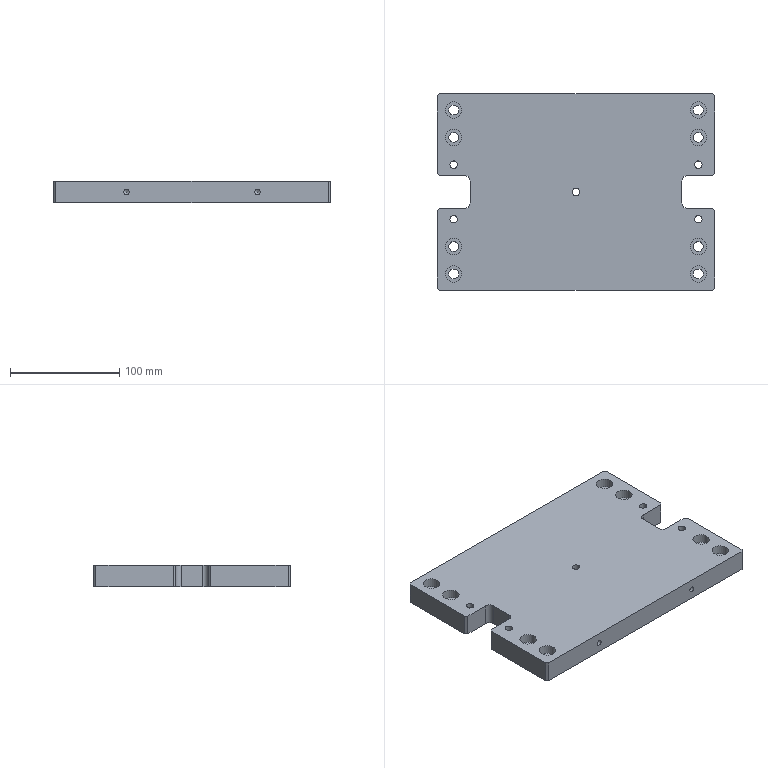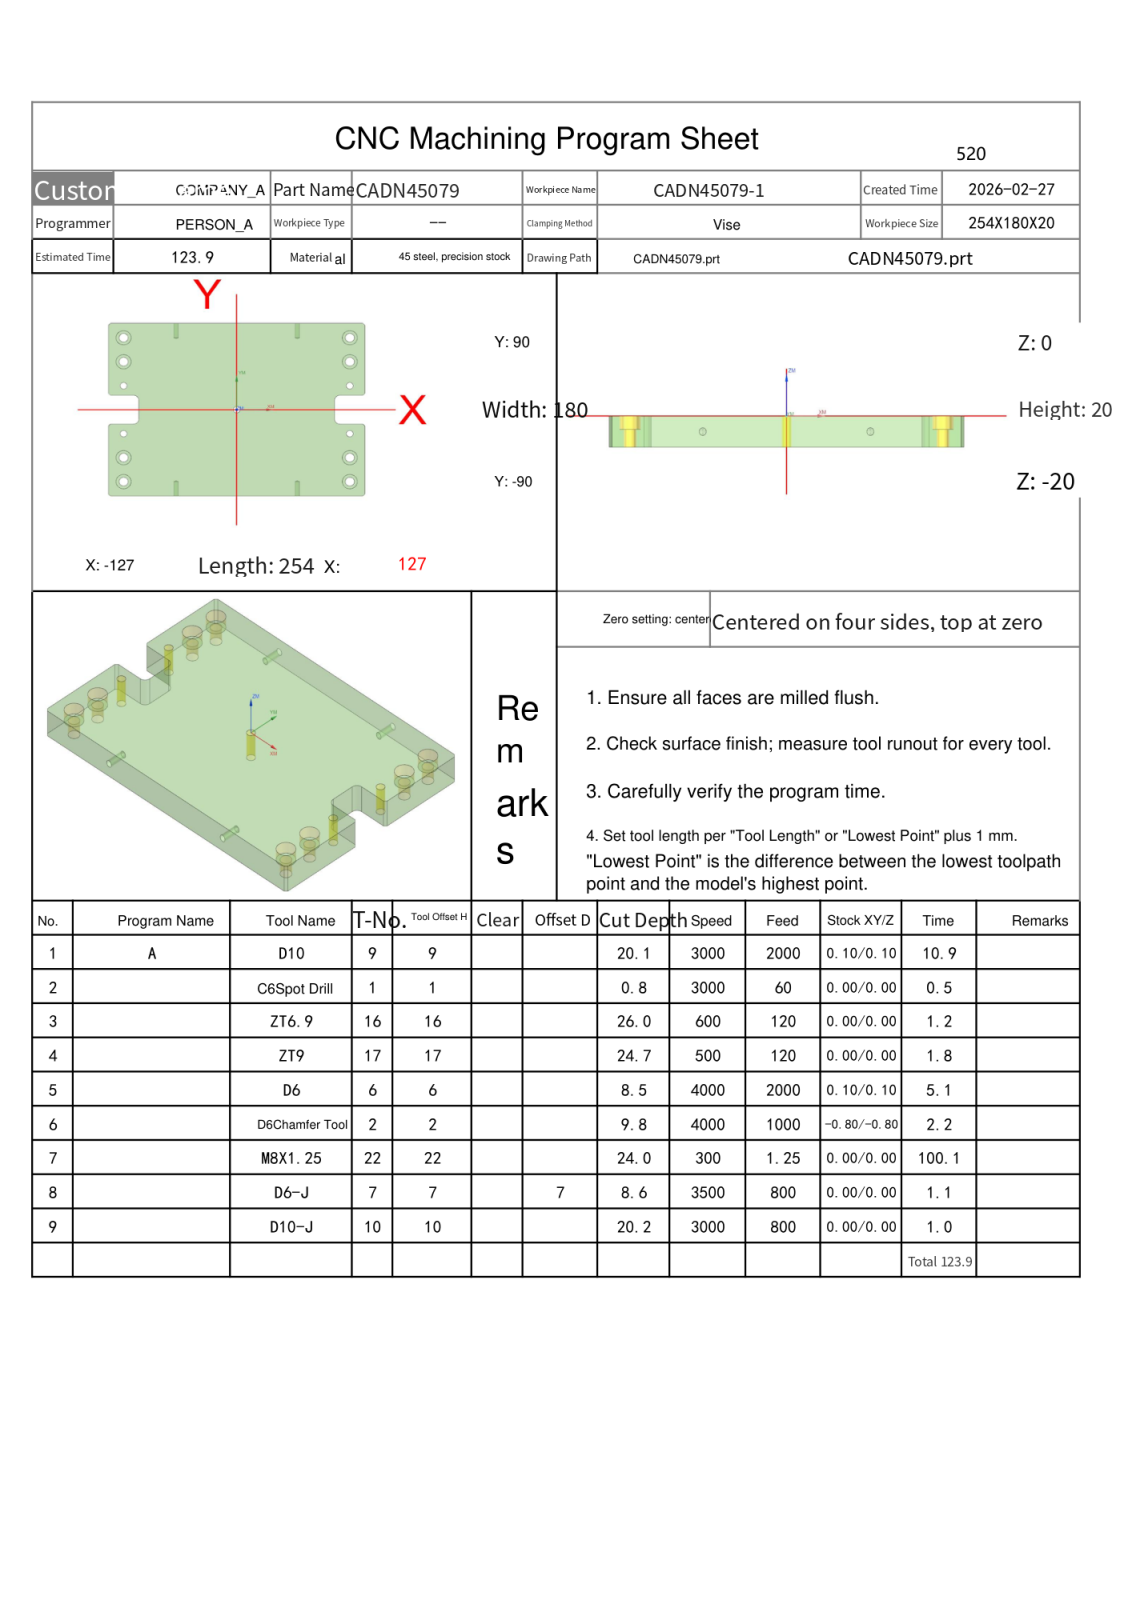NC program | NX | posted by the shop | part box 254 x 180 x 20 mm
Lines 2475 to 3296 of 5116:
N5 T06 M06
(D6  D=6. R=0. H=06 ce=0.10 di=0.10)
G00 G90 G54 X110.307 Y54.088 M03 S4000
G43 H06 Z30.
M08
Z1.
G01 X109.313 Y53.522 Z.94 F2000.
X108.478 Y52.687 Z.878
X107.893 Y51.66 Z.816
X107.6 Y50.515 Z.754
Y49.485 Z.7
X107.893 Y48.34 Z.638
X108.478 Y47.313 Z.576
X109.313 Y46.478 Z.514
X110.34 Y45.893 Z.453
X111.485 Y45.6 Z.391
X112.515 Z.337
X113.66 Y45.893 Z.275
X114.687 Y46.478 Z.213
X115.522 Y47.313 Z.151
X116.107 Y48.34 Z.089
X116.4 Y49.485 Z.027
Y50. Z0.0
G03 X112. Y54.4 Z-.049 I-4.4 J0.0
X107.6 Y50. Z-.099 I0.0 J-4.4
X112. Y45.6 Z-.148 I4.4 J0.0
X116.4 Y50. Z-.198 I0.0 J4.4
X112. Y54.4 Z-.247 I-4.4 J0.0
X107.6 Y50. Z-.297 I0.0 J-4.4
X112. Y45.6 Z-.346 I4.4 J0.0
X116.4 Y50. Z-.395 I0.0 J4.4
X112. Y54.4 Z-.445 I-4.4 J0.0
X107.6 Y50. Z-.494 I0.0 J-4.4
X112. Y45.6 Z-.544 I4.4 J0.0
X116.4 Y50. Z-.593 I0.0 J4.4
X112. Y54.4 Z-.642 I-4.4 J0.0
X107.6 Y50. Z-.692 I0.0 J-4.4
X112. Y45.6 Z-.741 I4.4 J0.0
X116.4 Y50. Z-.791 I0.0 J4.4
X112. Y54.4 Z-.84 I-4.4 J0.0
X107.6 Y50. Z-.89 I0.0 J-4.4
X112. Y45.6 Z-.939 I4.4 J0.0
X116.4 Y50. Z-.988 I0.0 J4.4
X112. Y54.4 Z-1.038 I-4.4 J0.0
X107.6 Y50. Z-1.087 I0.0 J-4.4
X112. Y45.6 Z-1.137 I4.4 J0.0
X116.4 Y50. Z-1.186 I0.0 J4.4
X112. Y54.4 Z-1.235 I-4.4 J0.0
X107.6 Y50. Z-1.285 I0.0 J-4.4
X112. Y45.6 Z-1.334 I4.4 J0.0
X116.4 Y50. Z-1.384 I0.0 J4.4
X112. Y54.4 Z-1.433 I-4.4 J0.0
X107.6 Y50. Z-1.483 I0.0 J-4.4
X112. Y45.6 Z-1.532 I4.4 J0.0
X116.4 Y50. Z-1.581 I0.0 J4.4
X112. Y54.4 Z-1.631 I-4.4 J0.0
X107.6 Y50. Z-1.68 I0.0 J-4.4
X112. Y45.6 Z-1.73 I4.4 J0.0
X116.4 Y50. Z-1.779 I0.0 J4.4
X112. Y54.4 Z-1.828 I-4.4 J0.0
X107.6 Y50. Z-1.878 I0.0 J-4.4
X112. Y45.6 Z-1.927 I4.4 J0.0
X116.4 Y50. Z-1.977 I0.0 J4.4
X112. Y54.4 Z-2.026 I-4.4 J0.0
X107.6 Y50. Z-2.076 I0.0 J-4.4
X112. Y45.6 Z-2.125 I4.4 J0.0
X116.4 Y50. Z-2.174 I0.0 J4.4
X112. Y54.4 Z-2.224 I-4.4 J0.0
X107.6 Y50. Z-2.273 I0.0 J-4.4
X112. Y45.6 Z-2.323 I4.4 J0.0
X116.4 Y50. Z-2.372 I0.0 J4.4
X112. Y54.4 Z-2.422 I-4.4 J0.0
X107.6 Y50. Z-2.471 I0.0 J-4.4
X112. Y45.6 Z-2.52 I4.4 J0.0
X116.4 Y50. Z-2.57 I0.0 J4.4
X112. Y54.4 Z-2.619 I-4.4 J0.0
X107.6 Y50. Z-2.669 I0.0 J-4.4
X112. Y45.6 Z-2.718 I4.4 J0.0
X116.4 Y50. Z-2.767 I0.0 J4.4
X112. Y54.4 Z-2.817 I-4.4 J0.0
X107.6 Y50. Z-2.866 I0.0 J-4.4
X112. Y45.6 Z-2.916 I4.4 J0.0
X116.4 Y50. Z-2.965 I0.0 J4.4
X112. Y54.4 Z-3.015 I-4.4 J0.0
X107.6 Y50. Z-3.064 I0.0 J-4.4
X112. Y45.6 Z-3.113 I4.4 J0.0
X116.4 Y50. Z-3.163 I0.0 J4.4
X112. Y54.4 Z-3.212 I-4.4 J0.0
X107.6 Y50. Z-3.262 I0.0 J-4.4
X112. Y45.6 Z-3.311 I4.4 J0.0
X116.4 Y50. Z-3.36 I0.0 J4.4
X112. Y54.4 Z-3.41 I-4.4 J0.0
X107.6 Y50. Z-3.459 I0.0 J-4.4
X112. Y45.6 Z-3.509 I4.4 J0.0
X116.4 Y50. Z-3.558 I0.0 J4.4
X112. Y54.4 Z-3.608 I-4.4 J0.0
X107.6 Y50. Z-3.657 I0.0 J-4.4
X112. Y45.6 Z-3.706 I4.4 J0.0
X116.4 Y50. Z-3.756 I0.0 J4.4
X112. Y54.4 Z-3.805 I-4.4 J0.0
X107.6 Y50. Z-3.855 I0.0 J-4.4
X112. Y45.6 Z-3.904 I4.4 J0.0
X116.4 Y50. Z-3.953 I0.0 J4.4
X112. Y54.4 Z-4.003 I-4.4 J0.0
X107.6 Y50. Z-4.052 I0.0 J-4.4
X112. Y45.6 Z-4.102 I4.4 J0.0
X116.4 Y50. Z-4.151 I0.0 J4.4
X112. Y54.4 Z-4.201 I-4.4 J0.0
X107.6 Y50. Z-4.25 I0.0 J-4.4
X112. Y45.6 Z-4.299 I4.4 J0.0
X116.4 Y50. Z-4.349 I0.0 J4.4
X112. Y54.4 Z-4.398 I-4.4 J0.0
X107.6 Y50. Z-4.448 I0.0 J-4.4
X112. Y45.6 Z-4.497 I4.4 J0.0
X116.4 Y50. Z-4.547 I0.0 J4.4
X112. Y54.4 Z-4.596 I-4.4 J0.0
X107.6 Y50. Z-4.645 I0.0 J-4.4
X112. Y45.6 Z-4.695 I4.4 J0.0
X116.4 Y50. Z-4.744 I0.0 J4.4
X112. Y54.4 Z-4.794 I-4.4 J0.0
X107.6 Y50. Z-4.843 I0.0 J-4.4
X112. Y45.6 Z-4.892 I4.4 J0.0
X116.4 Y50. Z-4.942 I0.0 J4.4
X112. Y54.4 Z-4.991 I-4.4 J0.0
X107.6 Y50. Z-5.041 I0.0 J-4.4
X112. Y45.6 Z-5.09 I4.4 J0.0
X116.4 Y50. Z-5.14 I0.0 J4.4
X112. Y54.4 Z-5.189 I-4.4 J0.0
X107.6 Y50. Z-5.238 I0.0 J-4.4
X112. Y45.6 Z-5.288 I4.4 J0.0
X116.4 Y50. Z-5.337 I0.0 J4.4
X112. Y54.4 Z-5.387 I-4.4 J0.0
X107.6 Y50. Z-5.436 I0.0 J-4.4
X112. Y45.6 Z-5.485 I4.4 J0.0
X116.4 Y50. Z-5.535 I0.0 J4.4
X112. Y54.4 Z-5.584 I-4.4 J0.0
X107.6 Y50. Z-5.634 I0.0 J-4.4
X112. Y45.6 Z-5.683 I4.4 J0.0
X116.4 Y50. Z-5.733 I0.0 J4.4
X112. Y54.4 Z-5.782 I-4.4 J0.0
X107.6 Y50. Z-5.831 I0.0 J-4.4
X112. Y45.6 Z-5.881 I4.4 J0.0
X116.4 Y50. Z-5.93 I0.0 J4.4
X112. Y54.4 Z-5.98 I-4.4 J0.0
X107.6 Y50. Z-6.029 I0.0 J-4.4
X112. Y45.6 Z-6.078 I4.4 J0.0
X116.4 Y50. Z-6.128 I0.0 J4.4
X112. Y54.4 Z-6.177 I-4.4 J0.0
X107.6 Y50. Z-6.227 I0.0 J-4.4
X112. Y45.6 Z-6.276 I4.4 J0.0
X116.4 Y50. Z-6.326 I0.0 J4.4
X112. Y54.4 Z-6.375 I-4.4 J0.0
X107.6 Y50. Z-6.424 I0.0 J-4.4
X112. Y45.6 Z-6.474 I4.4 J0.0
X116.4 Y50. Z-6.523 I0.0 J4.4
X112. Y54.4 Z-6.573 I-4.4 J0.0
X107.6 Y50. Z-6.622 I0.0 J-4.4
X112. Y45.6 Z-6.672 I4.4 J0.0
X116.4 Y50. Z-6.721 I0.0 J4.4
X112. Y54.4 Z-6.77 I-4.4 J0.0
X107.6 Y50. Z-6.82 I0.0 J-4.4
X112. Y45.6 Z-6.869 I4.4 J0.0
X116.4 Y50. Z-6.919 I0.0 J4.4
X112. Y54.4 Z-6.968 I-4.4 J0.0
X107.6 Y50. Z-7.017 I0.0 J-4.4
X112. Y45.6 Z-7.067 I4.4 J0.0
X116.4 Y50. Z-7.116 I0.0 J4.4
X112. Y54.4 Z-7.166 I-4.4 J0.0
X107.6 Y50. Z-7.215 I0.0 J-4.4
X112. Y45.6 Z-7.265 I4.4 J0.0
X116.4 Y50. Z-7.314 I0.0 J4.4
X112. Y54.4 Z-7.363 I-4.4 J0.0
X107.6 Y50. Z-7.413 I0.0 J-4.4
X112. Y45.6 Z-7.462 I4.4 J0.0
X116.4 Y50. Z-7.512 I0.0 J4.4
X112. Y54.4 Z-7.561 I-4.4 J0.0
X107.6 Y50. Z-7.61 I0.0 J-4.4
X112. Y45.6 Z-7.66 I4.4 J0.0
X116.4 Y50. Z-7.709 I0.0 J4.4
X112. Y54.4 Z-7.759 I-4.4 J0.0
X107.6 Y50. Z-7.808 I0.0 J-4.4
X112. Y45.6 Z-7.858 I4.4 J0.0
X116.4 Y50. Z-7.907 I0.0 J4.4
X112. Y54.4 Z-7.956 I-4.4 J0.0
X107.6 Y50. Z-8.006 I0.0 J-4.4
X112. Y45.6 Z-8.055 I4.4 J0.0
X116.4 Y50. Z-8.105 I0.0 J4.4
X112. Y54.4 Z-8.154 I-4.4 J0.0
X107.6 Y50. Z-8.203 I0.0 J-4.4
X112. Y45.6 Z-8.253 I4.4 J0.0
X116.4 Y50. Z-8.302 I0.0 J4.4
X112. Y54.4 Z-8.352 I-4.4 J0.0
X107.6 Y50. Z-8.401 I0.0 J-4.4
X112. Y45.6 Z-8.451 I4.4 J0.0
X116.4 Y50. Z-8.5 I0.0 J4.4
X112. Y54.4 I-4.4 J0.0
X107.6 Y50. I0.0 J-4.4
X112. Y45.6 I4.4 J0.0
X116.4 Y50. I0.0 J4.4
X116.382 Y50.399 I-4.4 J0.0
G01 Z-7.5
G00 Z30.
X110.307 Y79.088
Z1.
G01 X109.313 Y78.522 Z.94
X108.478 Y77.687 Z.878
X107.893 Y76.66 Z.816
X107.6 Y75.515 Z.754
Y74.485 Z.7
X107.893 Y73.34 Z.638
X108.478 Y72.313 Z.576
X109.313 Y71.478 Z.514
X110.34 Y70.893 Z.453
X111.485 Y70.6 Z.391
X112.515 Z.337
X113.66 Y70.893 Z.275
X114.687 Y71.478 Z.213
X115.522 Y72.313 Z.151
X116.107 Y73.34 Z.089
X116.4 Y74.485 Z.027
Y75. Z0.0
G03 X112. Y79.4 Z-.049 I-4.4 J0.0
X107.6 Y75. Z-.099 I0.0 J-4.4
X112. Y70.6 Z-.148 I4.4 J0.0
X116.4 Y75. Z-.198 I0.0 J4.4
X112. Y79.4 Z-.247 I-4.4 J0.0
X107.6 Y75. Z-.297 I0.0 J-4.4
X112. Y70.6 Z-.346 I4.4 J0.0
X116.4 Y75. Z-.395 I0.0 J4.4
X112. Y79.4 Z-.445 I-4.4 J0.0
X107.6 Y75. Z-.494 I0.0 J-4.4
X112. Y70.6 Z-.544 I4.4 J0.0
X116.4 Y75. Z-.593 I0.0 J4.4
X112. Y79.4 Z-.642 I-4.4 J0.0
X107.6 Y75. Z-.692 I0.0 J-4.4
X112. Y70.6 Z-.741 I4.4 J0.0
X116.4 Y75. Z-.791 I0.0 J4.4
X112. Y79.4 Z-.84 I-4.4 J0.0
X107.6 Y75. Z-.89 I0.0 J-4.4
X112. Y70.6 Z-.939 I4.4 J0.0
X116.4 Y75. Z-.988 I0.0 J4.4
X112. Y79.4 Z-1.038 I-4.4 J0.0
X107.6 Y75. Z-1.087 I0.0 J-4.4
X112. Y70.6 Z-1.137 I4.4 J0.0
X116.4 Y75. Z-1.186 I0.0 J4.4
X112. Y79.4 Z-1.235 I-4.4 J0.0
X107.6 Y75. Z-1.285 I0.0 J-4.4
X112. Y70.6 Z-1.334 I4.4 J0.0
X116.4 Y75. Z-1.384 I0.0 J4.4
X112. Y79.4 Z-1.433 I-4.4 J0.0
X107.6 Y75. Z-1.483 I0.0 J-4.4
X112. Y70.6 Z-1.532 I4.4 J0.0
X116.4 Y75. Z-1.581 I0.0 J4.4
X112. Y79.4 Z-1.631 I-4.4 J0.0
X107.6 Y75. Z-1.68 I0.0 J-4.4
X112. Y70.6 Z-1.73 I4.4 J0.0
X116.4 Y75. Z-1.779 I0.0 J4.4
X112. Y79.4 Z-1.828 I-4.4 J0.0
X107.6 Y75. Z-1.878 I0.0 J-4.4
X112. Y70.6 Z-1.927 I4.4 J0.0
X116.4 Y75. Z-1.977 I0.0 J4.4
X112. Y79.4 Z-2.026 I-4.4 J0.0
X107.6 Y75. Z-2.076 I0.0 J-4.4
X112. Y70.6 Z-2.125 I4.4 J0.0
X116.4 Y75. Z-2.174 I0.0 J4.4
X112. Y79.4 Z-2.224 I-4.4 J0.0
X107.6 Y75. Z-2.273 I0.0 J-4.4
X112. Y70.6 Z-2.323 I4.4 J0.0
X116.4 Y75. Z-2.372 I0.0 J4.4
X112. Y79.4 Z-2.422 I-4.4 J0.0
X107.6 Y75. Z-2.471 I0.0 J-4.4
X112. Y70.6 Z-2.52 I4.4 J0.0
X116.4 Y75. Z-2.57 I0.0 J4.4
X112. Y79.4 Z-2.619 I-4.4 J0.0
X107.6 Y75. Z-2.669 I0.0 J-4.4
X112. Y70.6 Z-2.718 I4.4 J0.0
X116.4 Y75. Z-2.767 I0.0 J4.4
X112. Y79.4 Z-2.817 I-4.4 J0.0
X107.6 Y75. Z-2.866 I0.0 J-4.4
X112. Y70.6 Z-2.916 I4.4 J0.0
X116.4 Y75. Z-2.965 I0.0 J4.4
X112. Y79.4 Z-3.015 I-4.4 J0.0
X107.6 Y75. Z-3.064 I0.0 J-4.4
X112. Y70.6 Z-3.113 I4.4 J0.0
X116.4 Y75. Z-3.163 I0.0 J4.4
X112. Y79.4 Z-3.212 I-4.4 J0.0
X107.6 Y75. Z-3.262 I0.0 J-4.4
X112. Y70.6 Z-3.311 I4.4 J0.0
X116.4 Y75. Z-3.36 I0.0 J4.4
X112. Y79.4 Z-3.41 I-4.4 J0.0
X107.6 Y75. Z-3.459 I0.0 J-4.4
X112. Y70.6 Z-3.509 I4.4 J0.0
X116.4 Y75. Z-3.558 I0.0 J4.4
X112. Y79.4 Z-3.608 I-4.4 J0.0
X107.6 Y75. Z-3.657 I0.0 J-4.4
X112. Y70.6 Z-3.706 I4.4 J0.0
X116.4 Y75. Z-3.756 I0.0 J4.4
X112. Y79.4 Z-3.805 I-4.4 J0.0
X107.6 Y75. Z-3.855 I0.0 J-4.4
X112. Y70.6 Z-3.904 I4.4 J0.0
X116.4 Y75. Z-3.953 I0.0 J4.4
X112. Y79.4 Z-4.003 I-4.4 J0.0
X107.6 Y75. Z-4.052 I0.0 J-4.4
X112. Y70.6 Z-4.102 I4.4 J0.0
X116.4 Y75. Z-4.151 I0.0 J4.4
X112. Y79.4 Z-4.201 I-4.4 J0.0
X107.6 Y75. Z-4.25 I0.0 J-4.4
X112. Y70.6 Z-4.299 I4.4 J0.0
X116.4 Y75. Z-4.349 I0.0 J4.4
X112. Y79.4 Z-4.398 I-4.4 J0.0
X107.6 Y75. Z-4.448 I0.0 J-4.4
X112. Y70.6 Z-4.497 I4.4 J0.0
X116.4 Y75. Z-4.547 I0.0 J4.4
X112. Y79.4 Z-4.596 I-4.4 J0.0
X107.6 Y75. Z-4.645 I0.0 J-4.4
X112. Y70.6 Z-4.695 I4.4 J0.0
X116.4 Y75. Z-4.744 I0.0 J4.4
X112. Y79.4 Z-4.794 I-4.4 J0.0
X107.6 Y75. Z-4.843 I0.0 J-4.4
X112. Y70.6 Z-4.892 I4.4 J0.0
X116.4 Y75. Z-4.942 I0.0 J4.4
X112. Y79.4 Z-4.991 I-4.4 J0.0
X107.6 Y75. Z-5.041 I0.0 J-4.4
X112. Y70.6 Z-5.09 I4.4 J0.0
X116.4 Y75. Z-5.14 I0.0 J4.4
X112. Y79.4 Z-5.189 I-4.4 J0.0
X107.6 Y75. Z-5.238 I0.0 J-4.4
X112. Y70.6 Z-5.288 I4.4 J0.0
X116.4 Y75. Z-5.337 I0.0 J4.4
X112. Y79.4 Z-5.387 I-4.4 J0.0
X107.6 Y75. Z-5.436 I0.0 J-4.4
X112. Y70.6 Z-5.485 I4.4 J0.0
X116.4 Y75. Z-5.535 I0.0 J4.4
X112. Y79.4 Z-5.584 I-4.4 J0.0
X107.6 Y75. Z-5.634 I0.0 J-4.4
X112. Y70.6 Z-5.683 I4.4 J0.0
X116.4 Y75. Z-5.733 I0.0 J4.4
X112. Y79.4 Z-5.782 I-4.4 J0.0
X107.6 Y75. Z-5.831 I0.0 J-4.4
X112. Y70.6 Z-5.881 I4.4 J0.0
X116.4 Y75. Z-5.93 I0.0 J4.4
X112. Y79.4 Z-5.98 I-4.4 J0.0
X107.6 Y75. Z-6.029 I0.0 J-4.4
X112. Y70.6 Z-6.078 I4.4 J0.0
X116.4 Y75. Z-6.128 I0.0 J4.4
X112. Y79.4 Z-6.177 I-4.4 J0.0
X107.6 Y75. Z-6.227 I0.0 J-4.4
X112. Y70.6 Z-6.276 I4.4 J0.0
X116.4 Y75. Z-6.326 I0.0 J4.4
X112. Y79.4 Z-6.375 I-4.4 J0.0
X107.6 Y75. Z-6.424 I0.0 J-4.4
X112. Y70.6 Z-6.474 I4.4 J0.0
X116.4 Y75. Z-6.523 I0.0 J4.4
X112. Y79.4 Z-6.573 I-4.4 J0.0
X107.6 Y75. Z-6.622 I0.0 J-4.4
X112. Y70.6 Z-6.672 I4.4 J0.0
X116.4 Y75. Z-6.721 I0.0 J4.4
X112. Y79.4 Z-6.77 I-4.4 J0.0
X107.6 Y75. Z-6.82 I0.0 J-4.4
X112. Y70.6 Z-6.869 I4.4 J0.0
X116.4 Y75. Z-6.919 I0.0 J4.4
X112. Y79.4 Z-6.968 I-4.4 J0.0
X107.6 Y75. Z-7.017 I0.0 J-4.4
X112. Y70.6 Z-7.067 I4.4 J0.0
X116.4 Y75. Z-7.116 I0.0 J4.4
X112. Y79.4 Z-7.166 I-4.4 J0.0
X107.6 Y75. Z-7.215 I0.0 J-4.4
X112. Y70.6 Z-7.265 I4.4 J0.0
X116.4 Y75. Z-7.314 I0.0 J4.4
X112. Y79.4 Z-7.363 I-4.4 J0.0
X107.6 Y75. Z-7.413 I0.0 J-4.4
X112. Y70.6 Z-7.462 I4.4 J0.0
X116.4 Y75. Z-7.512 I0.0 J4.4
X112. Y79.4 Z-7.561 I-4.4 J0.0
X107.6 Y75. Z-7.61 I0.0 J-4.4
X112. Y70.6 Z-7.66 I4.4 J0.0
X116.4 Y75. Z-7.709 I0.0 J4.4
X112. Y79.4 Z-7.759 I-4.4 J0.0
X107.6 Y75. Z-7.808 I0.0 J-4.4
X112. Y70.6 Z-7.858 I4.4 J0.0
X116.4 Y75. Z-7.907 I0.0 J4.4
X112. Y79.4 Z-7.956 I-4.4 J0.0
X107.6 Y75. Z-8.006 I0.0 J-4.4
X112. Y70.6 Z-8.055 I4.4 J0.0
X116.4 Y75. Z-8.105 I0.0 J4.4
X112. Y79.4 Z-8.154 I-4.4 J0.0
X107.6 Y75. Z-8.203 I0.0 J-4.4
X112. Y70.6 Z-8.253 I4.4 J0.0
X116.4 Y75. Z-8.302 I0.0 J4.4
X112. Y79.4 Z-8.352 I-4.4 J0.0
X107.6 Y75. Z-8.401 I0.0 J-4.4
X112. Y70.6 Z-8.451 I4.4 J0.0
X116.4 Y75. Z-8.5 I0.0 J4.4
X112. Y79.4 I-4.4 J0.0
X107.6 Y75. I0.0 J-4.4
X112. Y70.6 I4.4 J0.0
X116.4 Y75. I0.0 J4.4
X116.382 Y75.399 I-4.4 J0.0
G01 Z-7.5
G00 Z30.
X110.307 Y-70.912
Z1.
G01 X109.313 Y-71.478 Z.94
X108.478 Y-72.313 Z.878
X107.893 Y-73.34 Z.816
X107.6 Y-74.485 Z.754
Y-75.515 Z.7
X107.893 Y-76.66 Z.638
X108.478 Y-77.687 Z.576
X109.313 Y-78.522 Z.514
X110.34 Y-79.107 Z.453
X111.485 Y-79.4 Z.391
X112.515 Z.337
X113.66 Y-79.107 Z.275
X114.687 Y-78.522 Z.213
X115.522 Y-77.687 Z.151
X116.107 Y-76.66 Z.089
X116.4 Y-75.515 Z.027
Y-75. Z0.0
G03 X112. Y-70.6 Z-.049 I-4.4 J0.0
X107.6 Y-75. Z-.099 I0.0 J-4.4
X112. Y-79.4 Z-.148 I4.4 J0.0
X116.4 Y-75. Z-.198 I0.0 J4.4
X112. Y-70.6 Z-.247 I-4.4 J0.0
X107.6 Y-75. Z-.297 I0.0 J-4.4
X112. Y-79.4 Z-.346 I4.4 J0.0
X116.4 Y-75. Z-.395 I0.0 J4.4
X112. Y-70.6 Z-.445 I-4.4 J0.0
X107.6 Y-75. Z-.494 I0.0 J-4.4
X112. Y-79.4 Z-.544 I4.4 J0.0
X116.4 Y-75. Z-.593 I0.0 J4.4
X112. Y-70.6 Z-.642 I-4.4 J0.0
X107.6 Y-75. Z-.692 I0.0 J-4.4
X112. Y-79.4 Z-.741 I4.4 J0.0
X116.4 Y-75. Z-.791 I0.0 J4.4
X112. Y-70.6 Z-.84 I-4.4 J0.0
X107.6 Y-75. Z-.89 I0.0 J-4.4
X112. Y-79.4 Z-.939 I4.4 J0.0
X116.4 Y-75. Z-.988 I0.0 J4.4
X112. Y-70.6 Z-1.038 I-4.4 J0.0
X107.6 Y-75. Z-1.087 I0.0 J-4.4
X112. Y-79.4 Z-1.137 I4.4 J0.0
X116.4 Y-75. Z-1.186 I0.0 J4.4
X112. Y-70.6 Z-1.235 I-4.4 J0.0
X107.6 Y-75. Z-1.285 I0.0 J-4.4
X112. Y-79.4 Z-1.334 I4.4 J0.0
X116.4 Y-75. Z-1.384 I0.0 J4.4
X112. Y-70.6 Z-1.433 I-4.4 J0.0
X107.6 Y-75. Z-1.483 I0.0 J-4.4
X112. Y-79.4 Z-1.532 I4.4 J0.0
X116.4 Y-75. Z-1.581 I0.0 J4.4
X112. Y-70.6 Z-1.631 I-4.4 J0.0
X107.6 Y-75. Z-1.68 I0.0 J-4.4
X112. Y-79.4 Z-1.73 I4.4 J0.0
X116.4 Y-75. Z-1.779 I0.0 J4.4
X112. Y-70.6 Z-1.828 I-4.4 J0.0
X107.6 Y-75. Z-1.878 I0.0 J-4.4
X112. Y-79.4 Z-1.927 I4.4 J0.0
X116.4 Y-75. Z-1.977 I0.0 J4.4
X112. Y-70.6 Z-2.026 I-4.4 J0.0
X107.6 Y-75. Z-2.076 I0.0 J-4.4
X112. Y-79.4 Z-2.125 I4.4 J0.0
X116.4 Y-75. Z-2.174 I0.0 J4.4
X112. Y-70.6 Z-2.224 I-4.4 J0.0
X107.6 Y-75. Z-2.273 I0.0 J-4.4
X112. Y-79.4 Z-2.323 I4.4 J0.0
X116.4 Y-75. Z-2.372 I0.0 J4.4
X112. Y-70.6 Z-2.422 I-4.4 J0.0
X107.6 Y-75. Z-2.471 I0.0 J-4.4
X112. Y-79.4 Z-2.52 I4.4 J0.0
X116.4 Y-75. Z-2.57 I0.0 J4.4
X112. Y-70.6 Z-2.619 I-4.4 J0.0
X107.6 Y-75. Z-2.669 I0.0 J-4.4
X112. Y-79.4 Z-2.718 I4.4 J0.0
X116.4 Y-75. Z-2.767 I0.0 J4.4
X112. Y-70.6 Z-2.817 I-4.4 J0.0
X107.6 Y-75. Z-2.866 I0.0 J-4.4
X112. Y-79.4 Z-2.916 I4.4 J0.0
X116.4 Y-75. Z-2.965 I0.0 J4.4
X112. Y-70.6 Z-3.015 I-4.4 J0.0
X107.6 Y-75. Z-3.064 I0.0 J-4.4
X112. Y-79.4 Z-3.113 I4.4 J0.0
X116.4 Y-75. Z-3.163 I0.0 J4.4
X112. Y-70.6 Z-3.212 I-4.4 J0.0
X107.6 Y-75. Z-3.262 I0.0 J-4.4
X112. Y-79.4 Z-3.311 I4.4 J0.0
X116.4 Y-75. Z-3.36 I0.0 J4.4
X112. Y-70.6 Z-3.41 I-4.4 J0.0
X107.6 Y-75. Z-3.459 I0.0 J-4.4
X112. Y-79.4 Z-3.509 I4.4 J0.0
X116.4 Y-75. Z-3.558 I0.0 J4.4
X112. Y-70.6 Z-3.608 I-4.4 J0.0
X107.6 Y-75. Z-3.657 I0.0 J-4.4
X112. Y-79.4 Z-3.706 I4.4 J0.0
X116.4 Y-75. Z-3.756 I0.0 J4.4
X112. Y-70.6 Z-3.805 I-4.4 J0.0
X107.6 Y-75. Z-3.855 I0.0 J-4.4
X112. Y-79.4 Z-3.904 I4.4 J0.0
X116.4 Y-75. Z-3.953 I0.0 J4.4
X112. Y-70.6 Z-4.003 I-4.4 J0.0
X107.6 Y-75. Z-4.052 I0.0 J-4.4
X112. Y-79.4 Z-4.102 I4.4 J0.0
X116.4 Y-75. Z-4.151 I0.0 J4.4
X112. Y-70.6 Z-4.201 I-4.4 J0.0
X107.6 Y-75. Z-4.25 I0.0 J-4.4
X112. Y-79.4 Z-4.299 I4.4 J0.0
X116.4 Y-75. Z-4.349 I0.0 J4.4
X112. Y-70.6 Z-4.398 I-4.4 J0.0
X107.6 Y-75. Z-4.448 I0.0 J-4.4
X112. Y-79.4 Z-4.497 I4.4 J0.0
X116.4 Y-75. Z-4.547 I0.0 J4.4
X112. Y-70.6 Z-4.596 I-4.4 J0.0
X107.6 Y-75. Z-4.645 I0.0 J-4.4
X112. Y-79.4 Z-4.695 I4.4 J0.0
X116.4 Y-75. Z-4.744 I0.0 J4.4
X112. Y-70.6 Z-4.794 I-4.4 J0.0
X107.6 Y-75. Z-4.843 I0.0 J-4.4
X112. Y-79.4 Z-4.892 I4.4 J0.0
X116.4 Y-75. Z-4.942 I0.0 J4.4
X112. Y-70.6 Z-4.991 I-4.4 J0.0
X107.6 Y-75. Z-5.041 I0.0 J-4.4
X112. Y-79.4 Z-5.09 I4.4 J0.0
X116.4 Y-75. Z-5.14 I0.0 J4.4
X112. Y-70.6 Z-5.189 I-4.4 J0.0
X107.6 Y-75. Z-5.238 I0.0 J-4.4
X112. Y-79.4 Z-5.288 I4.4 J0.0
X116.4 Y-75. Z-5.337 I0.0 J4.4
X112. Y-70.6 Z-5.387 I-4.4 J0.0
X107.6 Y-75. Z-5.436 I0.0 J-4.4
X112. Y-79.4 Z-5.485 I4.4 J0.0
X116.4 Y-75. Z-5.535 I0.0 J4.4
X112. Y-70.6 Z-5.584 I-4.4 J0.0
X107.6 Y-75. Z-5.634 I0.0 J-4.4
X112. Y-79.4 Z-5.683 I4.4 J0.0
X116.4 Y-75. Z-5.733 I0.0 J4.4
X112. Y-70.6 Z-5.782 I-4.4 J0.0
X107.6 Y-75. Z-5.831 I0.0 J-4.4
X112. Y-79.4 Z-5.881 I4.4 J0.0
X116.4 Y-75. Z-5.93 I0.0 J4.4
X112. Y-70.6 Z-5.98 I-4.4 J0.0
X107.6 Y-75. Z-6.029 I0.0 J-4.4
X112. Y-79.4 Z-6.078 I4.4 J0.0
X116.4 Y-75. Z-6.128 I0.0 J4.4
X112. Y-70.6 Z-6.177 I-4.4 J0.0
X107.6 Y-75. Z-6.227 I0.0 J-4.4
X112. Y-79.4 Z-6.276 I4.4 J0.0
X116.4 Y-75. Z-6.326 I0.0 J4.4
X112. Y-70.6 Z-6.375 I-4.4 J0.0
X107.6 Y-75. Z-6.424 I0.0 J-4.4
X112. Y-79.4 Z-6.474 I4.4 J0.0
X116.4 Y-75. Z-6.523 I0.0 J4.4
X112. Y-70.6 Z-6.573 I-4.4 J0.0
X107.6 Y-75. Z-6.622 I0.0 J-4.4
X112. Y-79.4 Z-6.672 I4.4 J0.0
X116.4 Y-75. Z-6.721 I0.0 J4.4
X112. Y-70.6 Z-6.77 I-4.4 J0.0
X107.6 Y-75. Z-6.82 I0.0 J-4.4
X112. Y-79.4 Z-6.869 I4.4 J0.0
X116.4 Y-75. Z-6.919 I0.0 J4.4
X112. Y-70.6 Z-6.968 I-4.4 J0.0
X107.6 Y-75. Z-7.017 I0.0 J-4.4
X112. Y-79.4 Z-7.067 I4.4 J0.0
X116.4 Y-75. Z-7.116 I0.0 J4.4
X112. Y-70.6 Z-7.166 I-4.4 J0.0
X107.6 Y-75. Z-7.215 I0.0 J-4.4
X112. Y-79.4 Z-7.265 I4.4 J0.0
X116.4 Y-75. Z-7.314 I0.0 J4.4
X112. Y-70.6 Z-7.363 I-4.4 J0.0
X107.6 Y-75. Z-7.413 I0.0 J-4.4
X112. Y-79.4 Z-7.462 I4.4 J0.0
X116.4 Y-75. Z-7.512 I0.0 J4.4
X112. Y-70.6 Z-7.561 I-4.4 J0.0
X107.6 Y-75. Z-7.61 I0.0 J-4.4
X112. Y-79.4 Z-7.66 I4.4 J0.0
X116.4 Y-75. Z-7.709 I0.0 J4.4
X112. Y-70.6 Z-7.759 I-4.4 J0.0
X107.6 Y-75. Z-7.808 I0.0 J-4.4
X112. Y-79.4 Z-7.858 I4.4 J0.0
X116.4 Y-75. Z-7.907 I0.0 J4.4
X112. Y-70.6 Z-7.956 I-4.4 J0.0
X107.6 Y-75. Z-8.006 I0.0 J-4.4
X112. Y-79.4 Z-8.055 I4.4 J0.0
X116.4 Y-75. Z-8.105 I0.0 J4.4
X112. Y-70.6 Z-8.154 I-4.4 J0.0
X107.6 Y-75. Z-8.203 I0.0 J-4.4
X112. Y-79.4 Z-8.253 I4.4 J0.0
X116.4 Y-75. Z-8.302 I0.0 J4.4
X112. Y-70.6 Z-8.352 I-4.4 J0.0
X107.6 Y-75. Z-8.401 I0.0 J-4.4
X112. Y-79.4 Z-8.451 I4.4 J0.0
X116.4 Y-75. Z-8.5 I0.0 J4.4
X112. Y-70.6 I-4.4 J0.0
X107.6 Y-75. I0.0 J-4.4
X112. Y-79.4 I4.4 J0.0
X116.4 Y-75. I0.0 J4.4
X116.382 Y-74.601 I-4.4 J0.0
G01 Z-7.5
G00 Z30.
X110.307 Y-45.912
Z1.
G01 X109.313 Y-46.478 Z.94
X108.478 Y-47.313 Z.878
X107.893 Y-48.34 Z.816
X107.6 Y-49.485 Z.754
Y-50.515 Z.7
X107.893 Y-51.66 Z.638
X108.478 Y-52.687 Z.576
X109.313 Y-53.522 Z.514
X110.34 Y-54.107 Z.453
X111.485 Y-54.4 Z.391
X112.515 Z.337
X113.66 Y-54.107 Z.275
X114.687 Y-53.522 Z.213
X115.522 Y-52.687 Z.151
X116.107 Y-51.66 Z.089
X116.4 Y-50.515 Z.027
Y-50. Z0.0
G03 X112. Y-45.6 Z-.049 I-4.4 J0.0
X107.6 Y-50. Z-.099 I0.0 J-4.4
X112. Y-54.4 Z-.148 I4.4 J0.0
X116.4 Y-50. Z-.198 I0.0 J4.4
X112. Y-45.6 Z-.247 I-4.4 J0.0
X107.6 Y-50. Z-.297 I0.0 J-4.4
X112. Y-54.4 Z-.346 I4.4 J0.0
X116.4 Y-50. Z-.395 I0.0 J4.4
X112. Y-45.6 Z-.445 I-4.4 J0.0
X107.6 Y-50. Z-.494 I0.0 J-4.4
X112. Y-54.4 Z-.544 I4.4 J0.0
X116.4 Y-50. Z-.593 I0.0 J4.4
X112. Y-45.6 Z-.642 I-4.4 J0.0
X107.6 Y-50. Z-.692 I0.0 J-4.4
X112. Y-54.4 Z-.741 I4.4 J0.0
X116.4 Y-50. Z-.791 I0.0 J4.4
X112. Y-45.6 Z-.84 I-4.4 J0.0
X107.6 Y-50. Z-.89 I0.0 J-4.4
X112. Y-54.4 Z-.939 I4.4 J0.0
X116.4 Y-50. Z-.988 I0.0 J4.4
X112. Y-45.6 Z-1.038 I-4.4 J0.0
X107.6 Y-50. Z-1.087 I0.0 J-4.4
X112. Y-54.4 Z-1.137 I4.4 J0.0
X116.4 Y-50. Z-1.186 I0.0 J4.4
X112. Y-45.6 Z-1.235 I-4.4 J0.0
X107.6 Y-50. Z-1.285 I0.0 J-4.4
X112. Y-54.4 Z-1.334 I4.4 J0.0
X116.4 Y-50. Z-1.384 I0.0 J4.4
X112. Y-45.6 Z-1.433 I-4.4 J0.0
X107.6 Y-50. Z-1.483 I0.0 J-4.4
X112. Y-54.4 Z-1.532 I4.4 J0.0
X116.4 Y-50. Z-1.581 I0.0 J4.4
X112. Y-45.6 Z-1.631 I-4.4 J0.0
X107.6 Y-50. Z-1.68 I0.0 J-4.4
X112. Y-54.4 Z-1.73 I4.4 J0.0
X116.4 Y-50. Z-1.779 I0.0 J4.4
X112. Y-45.6 Z-1.828 I-4.4 J0.0
X107.6 Y-50. Z-1.878 I0.0 J-4.4
X112. Y-54.4 Z-1.927 I4.4 J0.0
X116.4 Y-50. Z-1.977 I0.0 J4.4
X112. Y-45.6 Z-2.026 I-4.4 J0.0
X107.6 Y-50. Z-2.076 I0.0 J-4.4
X112. Y-54.4 Z-2.125 I4.4 J0.0
X116.4 Y-50. Z-2.174 I0.0 J4.4
X112. Y-45.6 Z-2.224 I-4.4 J0.0
X107.6 Y-50. Z-2.273 I0.0 J-4.4
X112. Y-54.4 Z-2.323 I4.4 J0.0
X116.4 Y-50. Z-2.372 I0.0 J4.4
X112. Y-45.6 Z-2.422 I-4.4 J0.0
X107.6 Y-50. Z-2.471 I0.0 J-4.4
X112. Y-54.4 Z-2.52 I4.4 J0.0
X116.4 Y-50. Z-2.57 I0.0 J4.4
X112. Y-45.6 Z-2.619 I-4.4 J0.0
X107.6 Y-50. Z-2.669 I0.0 J-4.4
X112. Y-54.4 Z-2.718 I4.4 J0.0
X116.4 Y-50. Z-2.767 I0.0 J4.4
X112. Y-45.6 Z-2.817 I-4.4 J0.0
X107.6 Y-50. Z-2.866 I0.0 J-4.4
X112. Y-54.4 Z-2.916 I4.4 J0.0
X116.4 Y-50. Z-2.965 I0.0 J4.4
X112. Y-45.6 Z-3.015 I-4.4 J0.0
X107.6 Y-50. Z-3.064 I0.0 J-4.4
X112. Y-54.4 Z-3.113 I4.4 J0.0
X116.4 Y-50. Z-3.163 I0.0 J4.4
X112. Y-45.6 Z-3.212 I-4.4 J0.0
X107.6 Y-50. Z-3.262 I0.0 J-4.4
X112. Y-54.4 Z-3.311 I4.4 J0.0
X116.4 Y-50. Z-3.36 I0.0 J4.4
X112. Y-45.6 Z-3.41 I-4.4 J0.0
X107.6 Y-50. Z-3.459 I0.0 J-4.4
X112. Y-54.4 Z-3.509 I4.4 J0.0
X116.4 Y-50. Z-3.558 I0.0 J4.4
X112. Y-45.6 Z-3.608 I-4.4 J0.0
X107.6 Y-50. Z-3.657 I0.0 J-4.4
X112. Y-54.4 Z-3.706 I4.4 J0.0
X116.4 Y-50. Z-3.756 I0.0 J4.4
X112. Y-45.6 Z-3.805 I-4.4 J0.0
X107.6 Y-50. Z-3.855 I0.0 J-4.4
X112. Y-54.4 Z-3.904 I4.4 J0.0
X116.4 Y-50. Z-3.953 I0.0 J4.4
X112. Y-45.6 Z-4.003 I-4.4 J0.0
X107.6 Y-50. Z-4.052 I0.0 J-4.4
X112. Y-54.4 Z-4.102 I4.4 J0.0
X116.4 Y-50. Z-4.151 I0.0 J4.4
X112. Y-45.6 Z-4.201 I-4.4 J0.0
X107.6 Y-50. Z-4.25 I0.0 J-4.4
X112. Y-54.4 Z-4.299 I4.4 J0.0
X116.4 Y-50. Z-4.349 I0.0 J4.4
X112. Y-45.6 Z-4.398 I-4.4 J0.0
X107.6 Y-50. Z-4.448 I0.0 J-4.4
X112. Y-54.4 Z-4.497 I4.4 J0.0
X116.4 Y-50. Z-4.547 I0.0 J4.4
X112. Y-45.6 Z-4.596 I-4.4 J0.0
X107.6 Y-50. Z-4.645 I0.0 J-4.4
X112. Y-54.4 Z-4.695 I4.4 J0.0
X116.4 Y-50. Z-4.744 I0.0 J4.4
X112. Y-45.6 Z-4.794 I-4.4 J0.0
X107.6 Y-50. Z-4.843 I0.0 J-4.4
X112. Y-54.4 Z-4.892 I4.4 J0.0
X116.4 Y-50. Z-4.942 I0.0 J4.4
X112. Y-45.6 Z-4.991 I-4.4 J0.0
X107.6 Y-50. Z-5.041 I0.0 J-4.4
X112. Y-54.4 Z-5.09 I4.4 J0.0
X116.4 Y-50. Z-5.14 I0.0 J4.4
X112. Y-45.6 Z-5.189 I-4.4 J0.0
X107.6 Y-50. Z-5.238 I0.0 J-4.4
X112. Y-54.4 Z-5.288 I4.4 J0.0
X116.4 Y-50. Z-5.337 I0.0 J4.4
X112. Y-45.6 Z-5.387 I-4.4 J0.0
X107.6 Y-50. Z-5.436 I0.0 J-4.4
X112. Y-54.4 Z-5.485 I4.4 J0.0
X116.4 Y-50. Z-5.535 I0.0 J4.4
X112. Y-45.6 Z-5.584 I-4.4 J0.0
X107.6 Y-50. Z-5.634 I0.0 J-4.4
X112. Y-54.4 Z-5.683 I4.4 J0.0
X116.4 Y-50. Z-5.733 I0.0 J4.4
X112. Y-45.6 Z-5.782 I-4.4 J0.0
X107.6 Y-50. Z-5.831 I0.0 J-4.4
X112. Y-54.4 Z-5.881 I4.4 J0.0
X116.4 Y-50. Z-5.93 I0.0 J4.4
X112. Y-45.6 Z-5.98 I-4.4 J0.0
X107.6 Y-50. Z-6.029 I0.0 J-4.4
X112. Y-54.4 Z-6.078 I4.4 J0.0
X116.4 Y-50. Z-6.128 I0.0 J4.4
X112. Y-45.6 Z-6.177 I-4.4 J0.0
X107.6 Y-50. Z-6.227 I0.0 J-4.4
X112. Y-54.4 Z-6.276 I4.4 J0.0
X116.4 Y-50. Z-6.326 I0.0 J4.4
X112. Y-45.6 Z-6.375 I-4.4 J0.0
X107.6 Y-50. Z-6.424 I0.0 J-4.4
X112. Y-54.4 Z-6.474 I4.4 J0.0
X116.4 Y-50. Z-6.523 I0.0 J4.4
X112. Y-45.6 Z-6.573 I-4.4 J0.0
X107.6 Y-50. Z-6.622 I0.0 J-4.4
X112. Y-54.4 Z-6.672 I4.4 J0.0
X116.4 Y-50. Z-6.721 I0.0 J4.4
X112. Y-45.6 Z-6.77 I-4.4 J0.0
X107.6 Y-50. Z-6.82 I0.0 J-4.4
X112. Y-54.4 Z-6.869 I4.4 J0.0
X116.4 Y-50. Z-6.919 I0.0 J4.4
X112. Y-45.6 Z-6.968 I-4.4 J0.0
X107.6 Y-50. Z-7.017 I0.0 J-4.4
X112. Y-54.4 Z-7.067 I4.4 J0.0
X116.4 Y-50. Z-7.116 I0.0 J4.4
X112. Y-45.6 Z-7.166 I-4.4 J0.0
X107.6 Y-50. Z-7.215 I0.0 J-4.4
X112. Y-54.4 Z-7.265 I4.4 J0.0
X116.4 Y-50. Z-7.314 I0.0 J4.4
X112. Y-45.6 Z-7.363 I-4.4 J0.0
X107.6 Y-50. Z-7.413 I0.0 J-4.4
X112. Y-54.4 Z-7.462 I4.4 J0.0
X116.4 Y-50. Z-7.512 I0.0 J4.4
X112. Y-45.6 Z-7.561 I-4.4 J0.0
X107.6 Y-50. Z-7.61 I0.0 J-4.4
X112. Y-54.4 Z-7.66 I4.4 J0.0
X116.4 Y-50. Z-7.709 I0.0 J4.4
X112. Y-45.6 Z-7.759 I-4.4 J0.0
X107.6 Y-50. Z-7.808 I0.0 J-4.4
X112. Y-54.4 Z-7.858 I4.4 J0.0
X116.4 Y-50. Z-7.907 I0.0 J4.4
X112. Y-45.6 Z-7.956 I-4.4 J0.0
X107.6 Y-50. Z-8.006 I0.0 J-4.4
X112. Y-54.4 Z-8.055 I4.4 J0.0
X116.4 Y-50. Z-8.105 I0.0 J4.4
X112. Y-45.6 Z-8.154 I-4.4 J0.0
X107.6 Y-50. Z-8.203 I0.0 J-4.4
X112. Y-54.4 Z-8.253 I4.4 J0.0
X116.4 Y-50. Z-8.302 I0.0 J4.4
X112. Y-45.6 Z-8.352 I-4.4 J0.0
X107.6 Y-50. Z-8.401 I0.0 J-4.4
X112. Y-54.4 Z-8.451 I4.4 J0.0
X116.4 Y-50. Z-8.5 I0.0 J4.4
X112. Y-45.6 I-4.4 J0.0
X107.6 Y-50. I0.0 J-4.4
X112. Y-54.4 I4.4 J0.0
X116.4 Y-50. I0.0 J4.4
X116.382 Y-49.601 I-4.4 J0.0
G01 Z-7.5
G00 Z30.
X-110.307 Y-54.088
Z1.
G01 X-109.313 Y-53.522 Z.94
X-108.478 Y-52.687 Z.878
X-107.893 Y-51.66 Z.816
X-107.6 Y-50.515 Z.754
Y-49.485 Z.7
X-107.893 Y-48.34 Z.638
X-108.478 Y-47.313 Z.576
X-109.313 Y-46.478 Z.514
X-110.34 Y-45.893 Z.453
X-111.485 Y-45.6 Z.391
X-112.515 Z.337
X-113.66 Y-45.893 Z.275
X-114.687 Y-46.478 Z.213
X-115.522 Y-47.313 Z.151
X-116.107 Y-48.34 Z.089
X-116.4 Y-49.485 Z.027
Y-50. Z0.0
G03 X-112. Y-54.4 Z-.049 I4.4 J0.0
X-107.6 Y-50. Z-.099 I0.0 J4.4
X-112. Y-45.6 Z-.148 I-4.4 J0.0
X-116.4 Y-50. Z-.198 I0.0 J-4.4
X-112. Y-54.4 Z-.247 I4.4 J0.0
X-107.6 Y-50. Z-.297 I0.0 J4.4
X-112. Y-45.6 Z-.346 I-4.4 J0.0